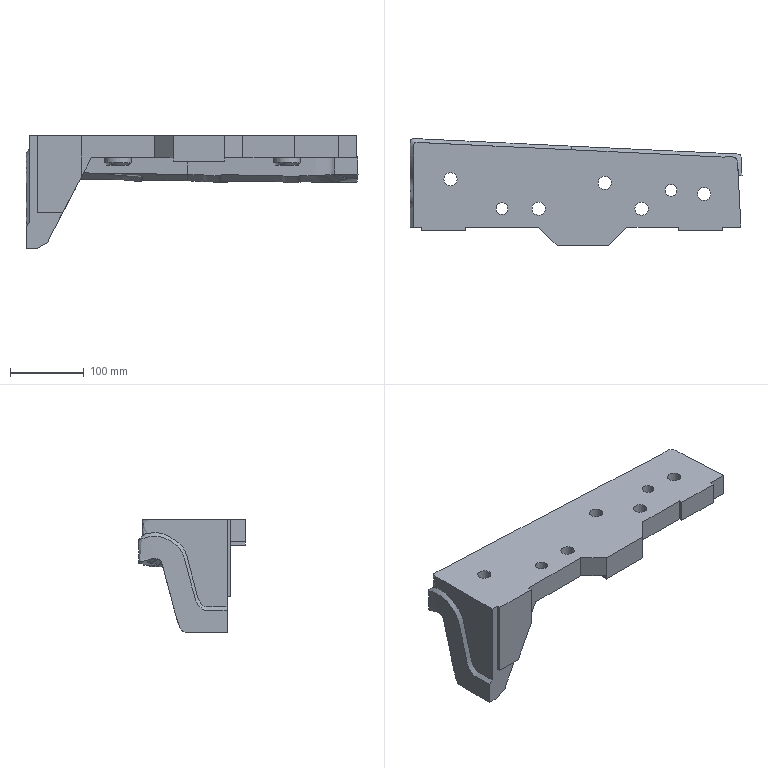Part | NX | features solid 2 | 1 solid | 65 faces | box 451.577 x 145.382 x 153.319 mm | volume 2216867 mm3 | plane 33 | spline 16 | cylinder 14 | cone 2 | commonest cylinder face diameters 18 x5 26 x5 16 x2 36 x2